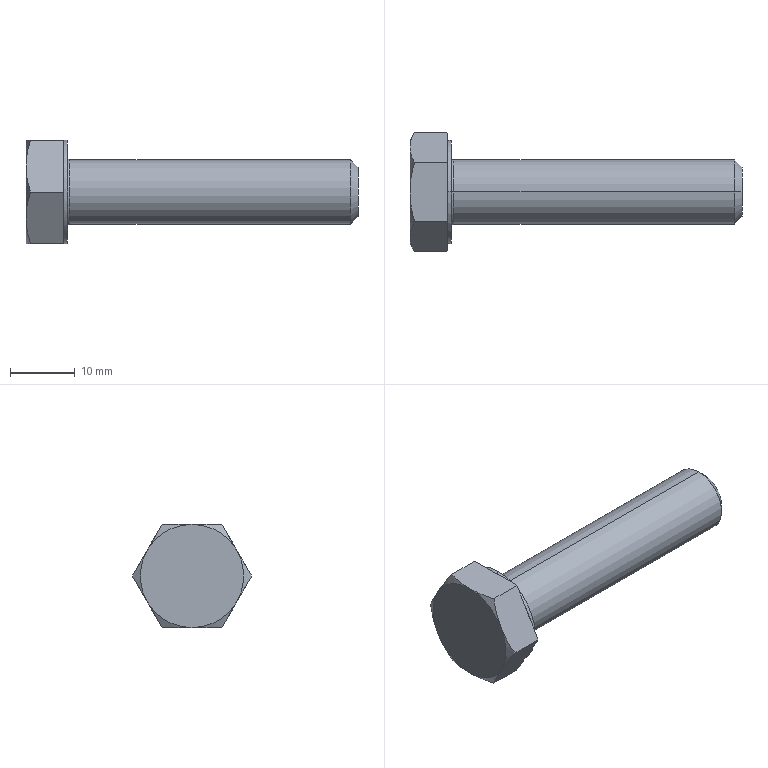Part | STEP file | GB/T5783-2000 hex head bolt, fully threaded M10×45 | 1 solid | 35 faces | box 51.4 x 18.475 x 16 mm | volume 4917 mm3 | plane 15 | cone 14 | cylinder 4 | torus 2 | commonest cylinder face diameters 10 x2 16 x2